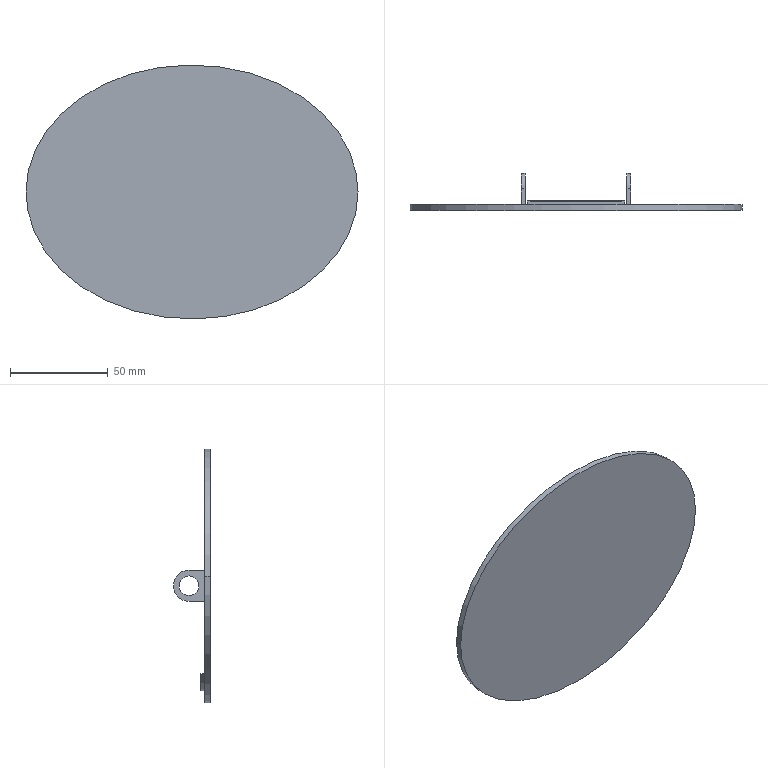Part | SolidWorks | features ICE 6, Extrusion 1, SweepCut 1 | 1 solid | 49 faces | box 170 x 19 x 130 mm | volume 53107 mm3 | plane 26 | cylinder 19 | spline 2 | torus 2 | commonest cylinder face diameters 1.5 x5 10 x4 16 x2 80 x2 74 x1 75 x1
STEP:
#1=CARTESIAN_POINT('',(0.,5.,-58.775));
#2=VERTEX_POINT('',#1);
#3=CARTESIAN_POINT('',(-25.,5.,-50.));
#4=VERTEX_POINT('',#3);
#5=CARTESIAN_POINT('',(0.,5.,-18.775));
#6=DIRECTION('',(0.,1.,0.));
#7=DIRECTION('',(0.,0.,-1.));
#8=AXIS2_PLACEMENT_3D('',#5,#6,#7);
#9=CIRCLE('',#8,40.);
#10=EDGE_CURVE('',#2,#4,#9,.T.);
#11=ORIENTED_EDGE('',*,*,#10,.F.);
#12=CARTESIAN_POINT('',(0.,3.,-58.775));
#13=VERTEX_POINT('',#12);
#14=CARTESIAN_POINT('',(0.,5.,-58.775));
#15=DIRECTION('',(0.,-1.,0.));
#16=VECTOR('',#15,1000.);
#17=LINE('',#14,#16);
#18=EDGE_CURVE('',#2,#13,#17,.T.);
#19=ORIENTED_EDGE('',*,*,#18,.T.);
#20=CARTESIAN_POINT('',(-25.,3.,-50.));
#21=VERTEX_POINT('',#20);
#22=CARTESIAN_POINT('',(0.,3.,-18.775));
#23=DIRECTION('',(0.,1.,0.));
#24=DIRECTION('',(0.,0.,-1.));
#25=AXIS2_PLACEMENT_3D('',#22,#23,#24);
#26=CIRCLE('',#25,40.);
#27=EDGE_CURVE('',#13,#21,#26,.T.);
#28=ORIENTED_EDGE('',*,*,#27,.T.);
#29=CARTESIAN_POINT('',(-25.,5.,-50.));
#30=DIRECTION('',(0.,-1.,0.));
#31=VECTOR('',#30,1000.);
#32=LINE('',#29,#31);
#33=EDGE_CURVE('',#4,#21,#32,.T.);
#34=ORIENTED_EDGE('',*,*,#33,.F.);
#35=EDGE_LOOP('',(#11,#19,#28,#34));
#36=FACE_OUTER_BOUND('',#35,.T.);
#37=CARTESIAN_POINT('',(0.,5.,-18.775));
#38=DIRECTION('',(0.,-1.,0.));
#39=DIRECTION('',(0.,0.,-1.));
#40=AXIS2_PLACEMENT_3D('',#37,#38,#39);
#41=CYLINDRICAL_SURFACE('',#40,40.);
#42=ADVANCED_FACE('',(#36),#41,.T.);
#43=CARTESIAN_POINT('',(-26.,11.,0.));
#44=VERTEX_POINT('',#43);
#45=CARTESIAN_POINT('',(-26.,11.,-10.));
#46=VERTEX_POINT('',#45);
#47=CARTESIAN_POINT('',(-26.,11.,-5.));
#48=DIRECTION('',(1.,0.,0.));
#49=DIRECTION('',(0.,0.,-1.));
#50=AXIS2_PLACEMENT_3D('',#47,#48,#49);
#51=CIRCLE('',#50,5.);
#52=EDGE_CURVE('',#44,#46,#51,.T.);
#53=ORIENTED_EDGE('',*,*,#52,.T.);
#54=CARTESIAN_POINT('',(-28.,11.,-10.));
#55=VERTEX_POINT('',#54);
#56=CARTESIAN_POINT('',(-26.,11.,-10.));
#57=DIRECTION('',(-1.,0.,0.));
#58=VECTOR('',#57,1000.);
#59=LINE('',#56,#58);
#60=EDGE_CURVE('',#46,#55,#59,.T.);
#61=ORIENTED_EDGE('',*,*,#60,.T.);
#62=CARTESIAN_POINT('',(-28.,11.,0.));
#63=VERTEX_POINT('',#62);
#64=CARTESIAN_POINT('',(-28.,11.,-5.));
#65=DIRECTION('',(1.,0.,0.));
#66=DIRECTION('',(0.,0.,-1.));
#67=AXIS2_PLACEMENT_3D('',#64,#65,#66);
#68=CIRCLE('',#67,5.);
#69=EDGE_CURVE('',#63,#55,#68,.T.);
#70=ORIENTED_EDGE('',*,*,#69,.F.);
#71=CARTESIAN_POINT('',(-26.,11.,0.));
#72=DIRECTION('',(-1.,0.,0.));
#73=VECTOR('',#72,1000.);
#74=LINE('',#71,#73);
#75=EDGE_CURVE('',#44,#63,#74,.T.);
#76=ORIENTED_EDGE('',*,*,#75,.F.);
#77=EDGE_LOOP('',(#53,#61,#70,#76));
#78=FACE_OUTER_BOUND('',#77,.T.);
#79=CARTESIAN_POINT('',(-26.,11.,-5.));
#80=DIRECTION('',(-1.,0.,0.));
#81=DIRECTION('',(0.,0.,1.));
#82=AXIS2_PLACEMENT_3D('',#79,#80,#81);
#83=CYLINDRICAL_SURFACE('',#82,5.);
#84=ADVANCED_FACE('',(#78),#83,.F.);
#85=CARTESIAN_POINT('',(26.,11.,0.));
#86=VERTEX_POINT('',#85);
#87=CARTESIAN_POINT('',(26.,11.,-10.));
#88=VERTEX_POINT('',#87);
#89=CARTESIAN_POINT('',(26.,11.,-5.));
#90=DIRECTION('',(1.,0.,0.));
#91=DIRECTION('',(0.,0.,-1.));
#92=AXIS2_PLACEMENT_3D('',#89,#90,#91);
#93=CIRCLE('',#92,5.);
#94=EDGE_CURVE('',#86,#88,#93,.T.);
#95=ORIENTED_EDGE('',*,*,#94,.F.);
#96=CARTESIAN_POINT('',(28.,11.,0.));
#97=VERTEX_POINT('',#96);
#98=CARTESIAN_POINT('',(26.,11.,0.));
#99=DIRECTION('',(1.,0.,0.));
#100=VECTOR('',#99,1000.);
#101=LINE('',#98,#100);
#102=EDGE_CURVE('',#86,#97,#101,.T.);
#103=ORIENTED_EDGE('',*,*,#102,.T.);
#104=CARTESIAN_POINT('',(28.,11.,-10.));
#105=VERTEX_POINT('',#104);
#106=CARTESIAN_POINT('',(28.,11.,-5.));
#107=DIRECTION('',(1.,0.,0.));
#108=DIRECTION('',(0.,0.,-1.));
#109=AXIS2_PLACEMENT_3D('',#106,#107,#108);
#110=CIRCLE('',#109,5.);
#111=EDGE_CURVE('',#97,#105,#110,.T.);
#112=ORIENTED_EDGE('',*,*,#111,.T.);
#113=CARTESIAN_POINT('',(26.,11.,-10.));
#114=DIRECTION('',(1.,0.,0.));
#115=VECTOR('',#114,1000.);
#116=LINE('',#113,#115);
#117=EDGE_CURVE('',#88,#105,#116,.T.);
#118=ORIENTED_EDGE('',*,*,#117,.F.);
#119=EDGE_LOOP('',(#95,#103,#112,#118));
#120=FACE_OUTER_BOUND('',#119,.T.);
#121=CARTESIAN_POINT('',(26.,11.,-5.));
#122=DIRECTION('',(1.,0.,0.));
#123=DIRECTION('',(0.,0.,-1.));
#124=AXIS2_PLACEMENT_3D('',#121,#122,#123);
#125=CYLINDRICAL_SURFACE('',#124,5.);
#126=ADVANCED_FACE('',(#120),#125,.F.);
#127=CARTESIAN_POINT('',(85.,3.,0.));
#128=VERTEX_POINT('',#127);
#129=CARTESIAN_POINT('',(-85.,3.,0.));
#130=VERTEX_POINT('',#129);
#131=CARTESIAN_POINT('',(85.,3.,0.));
#132=CARTESIAN_POINT('',(85.,3.,-130.));
#133=CARTESIAN_POINT('',(-85.,3.,-130.));
#134=CARTESIAN_POINT('',(-85.,3.,0.));
#135=(BOUNDED_CURVE()B_SPLINE_CURVE(3,(#131,#132,#133,#134),.UNSPECIFIED.,.F.,.T.)B_SPLINE_CURVE_WITH_KNOTS((4,4),(3.142,6.283),.UNSPECIFIED.)CURVE()GEOMETRIC_REPRESENTATION_ITEM()RATIONAL_B_SPLINE_CURVE((1.,0.3333,0.3333,1.))REPRESENTATION_ITEM(''));
#136=EDGE_CURVE('',#128,#130,#135,.T.);
#137=ORIENTED_EDGE('',*,*,#136,.F.);
#138=CARTESIAN_POINT('',(85.,0.,0.));
#139=VERTEX_POINT('',#138);
#140=CARTESIAN_POINT('',(85.,3.,0.));
#141=DIRECTION('',(0.,-1.,0.));
#142=VECTOR('',#141,1000.);
#143=LINE('',#140,#142);
#144=EDGE_CURVE('',#128,#139,#143,.T.);
#145=ORIENTED_EDGE('',*,*,#144,.T.);
#146=CARTESIAN_POINT('',(-85.,0.,0.));
#147=VERTEX_POINT('',#146);
#148=CARTESIAN_POINT('',(85.,0.,0.));
#149=CARTESIAN_POINT('',(85.,0.,-130.));
#150=CARTESIAN_POINT('',(-85.,0.,-130.));
#151=CARTESIAN_POINT('',(-85.,0.,0.));
#152=(BOUNDED_CURVE()B_SPLINE_CURVE(3,(#148,#149,#150,#151),.UNSPECIFIED.,.F.,.T.)B_SPLINE_CURVE_WITH_KNOTS((4,4),(3.142,6.283),.UNSPECIFIED.)CURVE()GEOMETRIC_REPRESENTATION_ITEM()RATIONAL_B_SPLINE_CURVE((1.,0.3333,0.3333,1.))REPRESENTATION_ITEM(''));
#153=EDGE_CURVE('',#139,#147,#152,.T.);
#154=ORIENTED_EDGE('',*,*,#153,.T.);
#155=CARTESIAN_POINT('',(-85.,3.,0.));
#156=DIRECTION('',(0.,-1.,0.));
#157=VECTOR('',#156,1000.);
#158=LINE('',#155,#157);
#159=EDGE_CURVE('',#130,#147,#158,.T.);
#160=ORIENTED_EDGE('',*,*,#159,.F.);
#161=EDGE_LOOP('',(#137,#145,#154,#160));
#162=FACE_OUTER_BOUND('',#161,.T.);
#163=CARTESIAN_POINT('',(85.,3.,0.));
#164=CARTESIAN_POINT('',(85.,0.,0.));
#165=CARTESIAN_POINT('',(85.,3.,-130.));
#166=CARTESIAN_POINT('',(85.,0.,-130.));
#167=CARTESIAN_POINT('',(-85.,3.,-130.));
#168=CARTESIAN_POINT('',(-85.,0.,-130.));
#169=CARTESIAN_POINT('',(-85.,3.,0.));
#170=CARTESIAN_POINT('',(-85.,0.,0.));
#171=(BOUNDED_SURFACE()B_SPLINE_SURFACE(3,1,((#163,#164),(#165,#166),(#167,#168),(#169,#170)),.UNSPECIFIED.,.F.,.F.,.T.)B_SPLINE_SURFACE_WITH_KNOTS((4,4),(2,2),(0.,1.),(0.,1.),.UNSPECIFIED.)GEOMETRIC_REPRESENTATION_ITEM()RATIONAL_B_SPLINE_SURFACE(((1.,1.),(0.3333,0.3333),(0.3333,0.3333),(1.,1.)))REPRESENTATION_ITEM('')SURFACE());
#172=ADVANCED_FACE('',(#162),#171,.F.);
#173=CARTESIAN_POINT('',(26.,3.,3.));
#174=VERTEX_POINT('',#173);
#175=CARTESIAN_POINT('',(26.,3.,-13.));
#176=VERTEX_POINT('',#175);
#177=CARTESIAN_POINT('',(26.,3.,-13.));
#178=DIRECTION('',(0.,0.,-1.));
#179=VECTOR('',#178,1000.);
#180=LINE('',#177,#179);
#181=EDGE_CURVE('',#174,#176,#180,.T.);
#182=ORIENTED_EDGE('',*,*,#181,.T.);
#183=CARTESIAN_POINT('',(28.,3.,-13.));
#184=VERTEX_POINT('',#183);
#185=CARTESIAN_POINT('',(26.,3.,-13.));
#186=DIRECTION('',(1.,0.,0.));
#187=VECTOR('',#186,1000.);
#188=LINE('',#185,#187);
#189=EDGE_CURVE('',#176,#184,#188,.T.);
#190=ORIENTED_EDGE('',*,*,#189,.T.);
#191=CARTESIAN_POINT('',(28.,3.,3.));
#192=VERTEX_POINT('',#191);
#193=CARTESIAN_POINT('',(28.,3.,-13.));
#194=DIRECTION('',(0.,0.,-1.));
#195=VECTOR('',#194,1000.);
#196=LINE('',#193,#195);
#197=EDGE_CURVE('',#192,#184,#196,.T.);
#198=ORIENTED_EDGE('',*,*,#197,.F.);
#199=CARTESIAN_POINT('',(26.,3.,3.));
#200=DIRECTION('',(1.,0.,0.));
#201=VECTOR('',#200,1000.);
#202=LINE('',#199,#201);
#203=EDGE_CURVE('',#174,#192,#202,.T.);
#204=ORIENTED_EDGE('',*,*,#203,.F.);
#205=EDGE_LOOP('',(#182,#190,#198,#204));
#206=FACE_BOUND('',#205,.T.);
#207=CARTESIAN_POINT('',(-85.,3.,0.));
#208=CARTESIAN_POINT('',(-85.,3.,130.));
#209=CARTESIAN_POINT('',(85.,3.,130.));
#210=CARTESIAN_POINT('',(85.,3.,0.));
#211=(BOUNDED_CURVE()B_SPLINE_CURVE(3,(#207,#208,#209,#210),.UNSPECIFIED.,.F.,.T.)B_SPLINE_CURVE_WITH_KNOTS((4,4),(0.,3.142),.UNSPECIFIED.)CURVE()GEOMETRIC_REPRESENTATION_ITEM()RATIONAL_B_SPLINE_CURVE((1.,0.3333,0.3333,1.))REPRESENTATION_ITEM(''));
#212=EDGE_CURVE('',#130,#128,#211,.T.);
#213=ORIENTED_EDGE('',*,*,#212,.T.);
#214=ORIENTED_EDGE('',*,*,#136,.T.);
#215=EDGE_LOOP('',(#213,#214));
#216=FACE_OUTER_BOUND('',#215,.T.);
#217=CARTESIAN_POINT('',(-28.,3.,3.));
#218=VERTEX_POINT('',#217);
#219=CARTESIAN_POINT('',(-28.,3.,-13.));
#220=VERTEX_POINT('',#219);
#221=CARTESIAN_POINT('',(-28.,3.,-13.));
#222=DIRECTION('',(0.,0.,-1.));
#223=VECTOR('',#222,1000.);
#224=LINE('',#221,#223);
#225=EDGE_CURVE('',#218,#220,#224,.T.);
#226=ORIENTED_EDGE('',*,*,#225,.T.);
#227=CARTESIAN_POINT('',(-26.,3.,-13.));
#228=VERTEX_POINT('',#227);
#229=CARTESIAN_POINT('',(-26.,3.,-13.));
#230=DIRECTION('',(-1.,0.,0.));
#231=VECTOR('',#230,1000.);
#232=LINE('',#229,#231);
#233=EDGE_CURVE('',#228,#220,#232,.T.);
#234=ORIENTED_EDGE('',*,*,#233,.F.);
#235=CARTESIAN_POINT('',(-26.,3.,3.));
#236=VERTEX_POINT('',#235);
#237=CARTESIAN_POINT('',(-26.,3.,-13.));
#238=DIRECTION('',(0.,0.,-1.));
#239=VECTOR('',#238,1000.);
#240=LINE('',#237,#239);
#241=EDGE_CURVE('',#236,#228,#240,.T.);
#242=ORIENTED_EDGE('',*,*,#241,.F.);
#243=CARTESIAN_POINT('',(-26.,3.,3.));
#244=DIRECTION('',(-1.,0.,0.));
#245=VECTOR('',#244,1000.);
#246=LINE('',#243,#245);
#247=EDGE_CURVE('',#236,#218,#246,.T.);
#248=ORIENTED_EDGE('',*,*,#247,.T.);
#249=EDGE_LOOP('',(#226,#234,#242,#248));
#250=FACE_BOUND('',#249,.T.);
#251=CARTESIAN_POINT('',(-15.75,3.,30.));
#252=VERTEX_POINT('',#251);
#253=CARTESIAN_POINT('',(-15.75,3.,-5.));
#254=VERTEX_POINT('',#253);
#255=CARTESIAN_POINT('',(-15.75,3.,-5.));
#256=DIRECTION('',(0.,0.,-1.));
#257=VECTOR('',#256,1000.);
#258=LINE('',#255,#257);
#259=EDGE_CURVE('',#252,#254,#258,.T.);
#260=ORIENTED_EDGE('',*,*,#259,.T.);
#261=CARTESIAN_POINT('',(-15.75,3.,-10.));
#262=VERTEX_POINT('',#261);
#263=CARTESIAN_POINT('',(-15.75,3.,-10.));
#264=DIRECTION('',(0.,0.,-1.));
#265=VECTOR('',#264,1000.);
#266=LINE('',#263,#265);
#267=EDGE_CURVE('',#254,#262,#266,.T.);
#268=ORIENTED_EDGE('',*,*,#267,.T.);
#269=CARTESIAN_POINT('',(-14.25,3.,-10.));
#270=VERTEX_POINT('',#269);
#271=CARTESIAN_POINT('',(0.,3.,-10.));
#272=DIRECTION('',(-1.,0.,0.));
#273=VECTOR('',#272,1000.);
#274=LINE('',#271,#273);
#275=EDGE_CURVE('',#270,#262,#274,.T.);
#276=ORIENTED_EDGE('',*,*,#275,.F.);
#277=CARTESIAN_POINT('',(-14.25,3.,-5.));
#278=VERTEX_POINT('',#277);
#279=CARTESIAN_POINT('',(-14.25,3.,-10.));
#280=DIRECTION('',(0.,0.,1.));
#281=VECTOR('',#280,1000.);
#282=LINE('',#279,#281);
#283=EDGE_CURVE('',#270,#278,#282,.T.);
#284=ORIENTED_EDGE('',*,*,#283,.T.);
#285=CARTESIAN_POINT('',(-14.25,3.,30.));
#286=VERTEX_POINT('',#285);
#287=CARTESIAN_POINT('',(-14.25,3.,-5.));
#288=DIRECTION('',(0.,0.,1.));
#289=VECTOR('',#288,1000.);
#290=LINE('',#287,#289);
#291=EDGE_CURVE('',#278,#286,#290,.T.);
#292=ORIENTED_EDGE('',*,*,#291,.T.);
#293=CARTESIAN_POINT('',(-10.,3.,34.25));
#294=VERTEX_POINT('',#293);
#295=CARTESIAN_POINT('',(-10.,3.,30.));
#296=DIRECTION('',(0.,1.,0.));
#297=DIRECTION('',(0.,0.,-1.));
#298=AXIS2_PLACEMENT_3D('',#295,#296,#297);
#299=CIRCLE('',#298,4.25);
#300=EDGE_CURVE('',#286,#294,#299,.T.);
#301=ORIENTED_EDGE('',*,*,#300,.T.);
#302=CARTESIAN_POINT('',(10.,3.,34.25));
#303=VERTEX_POINT('',#302);
#304=CARTESIAN_POINT('',(-10.,3.,34.25));
#305=DIRECTION('',(1.,0.,0.));
#306=VECTOR('',#305,1000.);
#307=LINE('',#304,#306);
#308=EDGE_CURVE('',#294,#303,#307,.T.);
#309=ORIENTED_EDGE('',*,*,#308,.T.);
#310=CARTESIAN_POINT('',(14.25,3.,30.));
#311=VERTEX_POINT('',#310);
#312=CARTESIAN_POINT('',(10.,3.,30.));
#313=DIRECTION('',(0.,1.,0.));
#314=DIRECTION('',(0.,0.,-1.));
#315=AXIS2_PLACEMENT_3D('',#312,#313,#314);
#316=CIRCLE('',#315,4.25);
#317=EDGE_CURVE('',#303,#311,#316,.T.);
#318=ORIENTED_EDGE('',*,*,#317,.T.);
#319=CARTESIAN_POINT('',(14.25,3.,-5.));
#320=VERTEX_POINT('',#319);
#321=CARTESIAN_POINT('',(14.25,3.,30.));
#322=DIRECTION('',(0.,0.,-1.));
#323=VECTOR('',#322,1000.);
#324=LINE('',#321,#323);
#325=EDGE_CURVE('',#311,#320,#324,.T.);
#326=ORIENTED_EDGE('',*,*,#325,.T.);
#327=CARTESIAN_POINT('',(14.25,3.,-10.));
#328=VERTEX_POINT('',#327);
#329=CARTESIAN_POINT('',(14.25,3.,-5.));
#330=DIRECTION('',(0.,0.,-1.));
#331=VECTOR('',#330,1000.);
#332=LINE('',#329,#331);
#333=EDGE_CURVE('',#320,#328,#332,.T.);
#334=ORIENTED_EDGE('',*,*,#333,.T.);
#335=CARTESIAN_POINT('',(15.75,3.,-10.));
#336=VERTEX_POINT('',#335);
#337=CARTESIAN_POINT('',(0.,3.,-10.));
#338=DIRECTION('',(1.,0.,0.));
#339=VECTOR('',#338,1000.);
#340=LINE('',#337,#339);
#341=EDGE_CURVE('',#328,#336,#340,.T.);
#342=ORIENTED_EDGE('',*,*,#341,.T.);
#343=CARTESIAN_POINT('',(15.75,3.,-5.));
#344=VERTEX_POINT('',#343);
#345=CARTESIAN_POINT('',(15.75,3.,-5.));
#346=DIRECTION('',(0.,0.,1.));
#347=VECTOR('',#346,1000.);
#348=LINE('',#345,#347);
#349=EDGE_CURVE('',#336,#344,#348,.T.);
#350=ORIENTED_EDGE('',*,*,#349,.T.);
#351=CARTESIAN_POINT('',(15.75,3.,30.));
#352=VERTEX_POINT('',#351);
#353=CARTESIAN_POINT('',(15.75,3.,30.));
#354=DIRECTION('',(0.,0.,1.));
#355=VECTOR('',#354,1000.);
#356=LINE('',#353,#355);
#357=EDGE_CURVE('',#344,#352,#356,.T.);
#358=ORIENTED_EDGE('',*,*,#357,.T.);
#359=CARTESIAN_POINT('',(10.,3.,35.75));
#360=VERTEX_POINT('',#359);
#361=CARTESIAN_POINT('',(10.,3.,30.));
#362=DIRECTION('',(0.,-1.,0.));
#363=DIRECTION('',(0.,0.,1.));
#364=AXIS2_PLACEMENT_3D('',#361,#362,#363);
#365=CIRCLE('',#364,5.75);
#366=EDGE_CURVE('',#352,#360,#365,.T.);
#367=ORIENTED_EDGE('',*,*,#366,.T.);
#368=CARTESIAN_POINT('',(-10.,3.,35.75));
#369=VERTEX_POINT('',#368);
#370=CARTESIAN_POINT('',(-10.,3.,35.75));
#371=DIRECTION('',(-1.,0.,0.));
#372=VECTOR('',#371,1000.);
#373=LINE('',#370,#372);
#374=EDGE_CURVE('',#360,#369,#373,.T.);
#375=ORIENTED_EDGE('',*,*,#374,.T.);
#376=CARTESIAN_POINT('',(-10.,3.,30.));
#377=DIRECTION('',(0.,-1.,0.));
#378=DIRECTION('',(0.,0.,1.));
#379=AXIS2_PLACEMENT_3D('',#376,#377,#378);
#380=CIRCLE('',#379,5.75);
#381=EDGE_CURVE('',#369,#252,#380,.T.);
#382=ORIENTED_EDGE('',*,*,#381,.T.);
#383=EDGE_LOOP('',(#260,#268,#276,#284,#292,#301,#309,#318,#326,#334,#342,#350,#358,#367,#375,#382));
#384=FACE_BOUND('',#383,.T.);
#385=CARTESIAN_POINT('',(25.,3.,-50.));
#386=VERTEX_POINT('',#385);
#387=CARTESIAN_POINT('',(-25.,3.,-50.));
#388=DIRECTION('',(1.,0.,0.));
#389=VECTOR('',#388,1000.);
#390=LINE('',#387,#389);
#391=EDGE_CURVE('',#21,#386,#390,.T.);
#392=ORIENTED_EDGE('',*,*,#391,.F.);
#393=ORIENTED_EDGE('',*,*,#27,.F.);
#394=CARTESIAN_POINT('',(0.,3.,-18.775));
#395=DIRECTION('',(0.,1.,0.));
#396=DIRECTION('',(0.,0.,-1.));
#397=AXIS2_PLACEMENT_3D('',#394,#395,#396);
#398=CIRCLE('',#397,40.);
#399=EDGE_CURVE('',#386,#13,#398,.T.);
#400=ORIENTED_EDGE('',*,*,#399,.F.);
#401=EDGE_LOOP('',(#392,#393,#400));
#402=FACE_BOUND('',#401,.T.);
#403=CARTESIAN_POINT('',(0.,3.,0.));
#404=DIRECTION('',(0.,1.,0.));
#405=DIRECTION('',(0.,0.,1.));
#406=AXIS2_PLACEMENT_3D('',#403,#404,#405);
#407=PLANE('',#406);
#408=ADVANCED_FACE('',(#206,#216,#250,#384,#402),#407,.T.);
#409=ORIENTED_EDGE('',*,*,#144,.F.);
#410=ORIENTED_EDGE('',*,*,#212,.F.);
#411=ORIENTED_EDGE('',*,*,#159,.T.);
#412=CARTESIAN_POINT('',(-85.,0.,0.));
#413=CARTESIAN_POINT('',(-85.,0.,130.));
#414=CARTESIAN_POINT('',(85.,0.,130.));
#415=CARTESIAN_POINT('',(85.,0.,0.));
#416=(BOUNDED_CURVE()B_SPLINE_CURVE(3,(#412,#413,#414,#415),.UNSPECIFIED.,.F.,.F.)B_SPLINE_CURVE_WITH_KNOTS((4,4),(0.,3.142),.UNSPECIFIED.)CURVE()GEOMETRIC_REPRESENTATION_ITEM()RATIONAL_B_SPLINE_CURVE((1.,0.3333,0.3333,1.))REPRESENTATION_ITEM(''));
#417=EDGE_CURVE('',#147,#139,#416,.T.);
#418=ORIENTED_EDGE('',*,*,#417,.T.);
#419=EDGE_LOOP('',(#409,#410,#411,#418));
#420=FACE_OUTER_BOUND('',#419,.T.);
#421=CARTESIAN_POINT('',(-85.,3.,0.));
#422=CARTESIAN_POINT('',(-85.,0.,0.));
#423=CARTESIAN_POINT('',(-85.,3.,130.));
#424=CARTESIAN_POINT('',(-85.,0.,130.));
#425=CARTESIAN_POINT('',(85.,3.,130.));
#426=CARTESIAN_POINT('',(85.,0.,130.));
#427=CARTESIAN_POINT('',(85.,3.,0.));
#428=CARTESIAN_POINT('',(85.,0.,0.));
#429=(BOUNDED_SURFACE()B_SPLINE_SURFACE(3,1,((#421,#422),(#423,#424),(#425,#426),(#427,#428)),.UNSPECIFIED.,.F.,.F.,.T.)B_SPLINE_SURFACE_WITH_KNOTS((4,4),(2,2),(0.,1.),(0.,1.),.UNSPECIFIED.)GEOMETRIC_REPRESENTATION_ITEM()RATIONAL_B_SPLINE_SURFACE(((1.,1.),(0.3333,0.3333),(0.3333,0.3333),(1.,1.)))REPRESENTATION_ITEM('')SURFACE());
#430=ADVANCED_FACE('',(#420),#429,.F.);
#431=ORIENTED_EDGE('',*,*,#417,.F.);
#432=ORIENTED_EDGE('',*,*,#153,.F.);
#433=EDGE_LOOP('',(#431,#432));
#434=FACE_OUTER_BOUND('',#433,.T.);
#435=CARTESIAN_POINT('',(0.,0.,0.));
#436=DIRECTION('',(0.,1.,0.));
#437=DIRECTION('',(0.,0.,1.));
#438=AXIS2_PLACEMENT_3D('',#435,#436,#437);
#439=PLANE('',#438);
#440=ADVANCED_FACE('',(#434),#439,.F.);
#441=CARTESIAN_POINT('',(28.,11.,3.));
#442=VERTEX_POINT('',#441);
#443=CARTESIAN_POINT('',(28.,3.,3.));
#444=DIRECTION('',(0.,-1.,0.));
#445=VECTOR('',#444,1000.);
#446=LINE('',#443,#445);
#447=EDGE_CURVE('',#442,#192,#446,.T.);
#448=ORIENTED_EDGE('',*,*,#447,.F.);
#449=CARTESIAN_POINT('',(26.,11.,3.));
#450=VERTEX_POINT('',#449);
#451=CARTESIAN_POINT('',(26.,11.,3.));
#452=DIRECTION('',(1.,0.,0.));
#453=VECTOR('',#452,1000.);
#454=LINE('',#451,#453);
#455=EDGE_CURVE('',#450,#442,#454,.T.);
#456=ORIENTED_EDGE('',*,*,#455,.F.);
#457=CARTESIAN_POINT('',(26.,3.,3.));
#458=DIRECTION('',(0.,-1.,0.));
#459=VECTOR('',#458,1000.);
#460=LINE('',#457,#459);
#461=EDGE_CURVE('',#450,#174,#460,.T.);
#462=ORIENTED_EDGE('',*,*,#461,.T.);
#463=ORIENTED_EDGE('',*,*,#203,.T.);
#464=EDGE_LOOP('',(#448,#456,#462,#463));
#465=FACE_OUTER_BOUND('',#464,.T.);
#466=CARTESIAN_POINT('',(26.,3.,3.));
#467=DIRECTION('',(0.,0.,1.));
#468=DIRECTION('',(1.,0.,0.));
#469=AXIS2_PLACEMENT_3D('',#466,#467,#468);
#470=PLANE('',#469);
#471=ADVANCED_FACE('',(#465),#470,.T.);
#472=CARTESIAN_POINT('',(28.,11.,-13.));
#473=VERTEX_POINT('',#472);
#474=CARTESIAN_POINT('',(28.,11.,-5.));
#475=DIRECTION('',(1.,0.,0.));
#476=DIRECTION('',(0.,0.,1.));
#477=AXIS2_PLACEMENT_3D('',#474,#475,#476);
#478=CIRCLE('',#477,8.);
#479=EDGE_CURVE('',#473,#442,#478,.T.);
#480=ORIENTED_EDGE('',*,*,#479,.F.);
#481=CARTESIAN_POINT('',(26.,11.,-13.));
#482=VERTEX_POINT('',#481);
#483=CARTESIAN_POINT('',(26.,11.,-13.));
#484=DIRECTION('',(1.,0.,0.));
#485=VECTOR('',#484,1000.);
#486=LINE('',#483,#485);
#487=EDGE_CURVE('',#482,#473,#486,.T.);
#488=ORIENTED_EDGE('',*,*,#487,.F.);
#489=CARTESIAN_POINT('',(26.,11.,-5.));
#490=DIRECTION('',(1.,0.,0.));
#491=DIRECTION('',(0.,0.,1.));
#492=AXIS2_PLACEMENT_3D('',#489,#490,#491);
#493=CIRCLE('',#492,8.);
#494=EDGE_CURVE('',#482,#450,#493,.T.);
#495=ORIENTED_EDGE('',*,*,#494,.T.);
#496=ORIENTED_EDGE('',*,*,#455,.T.);
#497=EDGE_LOOP('',(#480,#488,#495,#496));
#498=FACE_OUTER_BOUND('',#497,.T.);
#499=CARTESIAN_POINT('',(26.,11.,-5.));
#500=DIRECTION('',(1.,0.,0.));
#501=DIRECTION('',(0.,0.,-1.));
#502=AXIS2_PLACEMENT_3D('',#499,#500,#501);
#503=CYLINDRICAL_SURFACE('',#502,8.);
#504=ADVANCED_FACE('',(#498),#503,.T.);
#505=CARTESIAN_POINT('',(28.,11.,-13.));
#506=DIRECTION('',(0.,1.,0.));
#507=VECTOR('',#506,1000.);
#508=LINE('',#505,#507);
#509=EDGE_CURVE('',#184,#473,#508,.T.);
#510=ORIENTED_EDGE('',*,*,#509,.F.);
#511=ORIENTED_EDGE('',*,*,#189,.F.);
#512=CARTESIAN_POINT('',(26.,11.,-13.));
#513=DIRECTION('',(0.,1.,0.));
#514=VECTOR('',#513,1000.);
#515=LINE('',#512,#514);
#516=EDGE_CURVE('',#176,#482,#515,.T.);
#517=ORIENTED_EDGE('',*,*,#516,.T.);
#518=ORIENTED_EDGE('',*,*,#487,.T.);
#519=EDGE_LOOP('',(#510,#511,#517,#518));
#520=FACE_OUTER_BOUND('',#519,.T.);
#521=CARTESIAN_POINT('',(26.,11.,-13.));
#522=DIRECTION('',(0.,0.,-1.));
#523=DIRECTION('',(-1.,0.,0.));
#524=AXIS2_PLACEMENT_3D('',#521,#522,#523);
#525=PLANE('',#524);
#526=ADVANCED_FACE('',(#520),#525,.T.);
#527=CARTESIAN_POINT('',(26.,11.,-5.));
#528=DIRECTION('',(1.,0.,0.));
#529=DIRECTION('',(0.,0.,-1.));
#530=AXIS2_PLACEMENT_3D('',#527,#528,#529);
#531=CIRCLE('',#530,5.);
#532=EDGE_CURVE('',#88,#86,#531,.T.);
#533=ORIENTED_EDGE('',*,*,#532,.T.);
#534=ORIENTED_EDGE('',*,*,#94,.T.);
#535=EDGE_LOOP('',(#533,#534));
#536=FACE_BOUND('',#535,.T.);
#537=ORIENTED_EDGE('',*,*,#181,.F.);
#538=ORIENTED_EDGE('',*,*,#461,.F.);
#539=ORIENTED_EDGE('',*,*,#494,.F.);
#540=ORIENTED_EDGE('',*,*,#516,.F.);
#541=EDGE_LOOP('',(#537,#538,#539,#540));
#542=FACE_OUTER_BOUND('',#541,.T.);
#543=CARTESIAN_POINT('',(26.,11.,-5.));
#544=DIRECTION('',(-1.,0.,0.));
#545=DIRECTION('',(0.,0.,1.));
#546=AXIS2_PLACEMENT_3D('',#543,#544,#545);
#547=PLANE('',#546);
#548=ADVANCED_FACE('',(#536,#542),#547,.T.);
#549=CARTESIAN_POINT('',(28.,11.,-5.));
#550=DIRECTION('',(1.,0.,0.));
#551=DIRECTION('',(0.,0.,-1.));
#552=AXIS2_PLACEMENT_3D('',#549,#550,#551);
#553=CIRCLE('',#552,5.);
#554=EDGE_CURVE('',#105,#97,#553,.T.);
#555=ORIENTED_EDGE('',*,*,#554,.F.);
#556=ORIENTED_EDGE('',*,*,#111,.F.);
#557=EDGE_LOOP('',(#555,#556));
#558=FACE_BOUND('',#557,.T.);
#559=ORIENTED_EDGE('',*,*,#197,.T.);
#560=ORIENTED_EDGE('',*,*,#509,.T.);
#561=ORIENTED_EDGE('',*,*,#479,.T.);
#562=ORIENTED_EDGE('',*,*,#447,.T.);
#563=EDGE_LOOP('',(#559,#560,#561,#562));
#564=FACE_OUTER_BOUND('',#563,.T.);
#565=CARTESIAN_POINT('',(28.,11.,-5.));
#566=DIRECTION('',(-1.,0.,0.));
#567=DIRECTION('',(0.,0.,1.));
#568=AXIS2_PLACEMENT_3D('',#565,#566,#567);
#569=PLANE('',#568);
#570=ADVANCED_FACE('',(#558,#564),#569,.F.);
#571=ORIENTED_EDGE('',*,*,#102,.F.);
#572=ORIENTED_EDGE('',*,*,#532,.F.);
#573=ORIENTED_EDGE('',*,*,#117,.T.);
#574=ORIENTED_EDGE('',*,*,#554,.T.);
#575=EDGE_LOOP('',(#571,#572,#573,#574));
#576=FACE_OUTER_BOUND('',#575,.T.);
#577=CARTESIAN_POINT('',(26.,11.,-5.));
#578=DIRECTION('',(1.,0.,0.));
#579=DIRECTION('',(0.,0.,-1.));
#580=AXIS2_PLACEMENT_3D('',#577,#578,#579);
#581=CYLINDRICAL_SURFACE('',#580,5.);
#582=ADVANCED_FACE('',(#576),#581,.F.);
#583=ORIENTED_EDGE('',*,*,#241,.T.);
#584=CARTESIAN_POINT('',(-26.,11.,-13.));
#585=VERTEX_POINT('',#584);
#586=CARTESIAN_POINT('',(-26.,11.,-13.));
#587=DIRECTION('',(0.,1.,0.));
#588=VECTOR('',#587,1000.);
#589=LINE('',#586,#588);
#590=EDGE_CURVE('',#228,#585,#589,.T.);
#591=ORIENTED_EDGE('',*,*,#590,.T.);
#592=CARTESIAN_POINT('',(-26.,11.,3.));
#593=VERTEX_POINT('',#592);
#594=CARTESIAN_POINT('',(-26.,11.,-5.));
#595=DIRECTION('',(1.,0.,0.));
#596=DIRECTION('',(0.,0.,1.));
#597=AXIS2_PLACEMENT_3D('',#594,#595,#596);
#598=CIRCLE('',#597,8.);
#599=EDGE_CURVE('',#585,#593,#598,.T.);
#600=ORIENTED_EDGE('',*,*,#599,.T.);
#601=CARTESIAN_POINT('',(-26.,3.,3.));
#602=DIRECTION('',(0.,-1.,0.));
#603=VECTOR('',#602,1000.);
#604=LINE('',#601,#603);
#605=EDGE_CURVE('',#593,#236,#604,.T.);
#606=ORIENTED_EDGE('',*,*,#605,.T.);
#607=EDGE_LOOP('',(#583,#591,#600,#606));
#608=FACE_OUTER_BOUND('',#607,.T.);
#609=ORIENTED_EDGE('',*,*,#52,.F.);
#610=CARTESIAN_POINT('',(-26.,11.,-5.));
#611=DIRECTION('',(1.,0.,0.));
#612=DIRECTION('',(0.,0.,-1.));
#613=AXIS2_PLACEMENT_3D('',#610,#611,#612);
#614=CIRCLE('',#613,5.);
#615=EDGE_CURVE('',#46,#44,#614,.T.);
#616=ORIENTED_EDGE('',*,*,#615,.F.);
#617=EDGE_LOOP('',(#609,#616));
#618=FACE_BOUND('',#617,.T.);
#619=CARTESIAN_POINT('',(-26.,11.,-5.));
#620=DIRECTION('',(-1.,0.,0.));
#621=DIRECTION('',(0.,0.,1.));
#622=AXIS2_PLACEMENT_3D('',#619,#620,#621);
#623=PLANE('',#622);
#624=ADVANCED_FACE('',(#608,#618),#623,.F.);
#625=ORIENTED_EDGE('',*,*,#225,.F.);
#626=CARTESIAN_POINT('',(-28.,11.,3.));
#627=VERTEX_POINT('',#626);
#628=CARTESIAN_POINT('',(-28.,3.,3.));
#629=DIRECTION('',(0.,-1.,0.));
#630=VECTOR('',#629,1000.);
#631=LINE('',#628,#630);
#632=EDGE_CURVE('',#627,#218,#631,.T.);
#633=ORIENTED_EDGE('',*,*,#632,.F.);
#634=CARTESIAN_POINT('',(-28.,11.,-13.));
#635=VERTEX_POINT('',#634);
#636=CARTESIAN_POINT('',(-28.,11.,-5.));
#637=DIRECTION('',(1.,0.,0.));
#638=DIRECTION('',(0.,0.,1.));
#639=AXIS2_PLACEMENT_3D('',#636,#637,#638);
#640=CIRCLE('',#639,8.);
#641=EDGE_CURVE('',#635,#627,#640,.T.);
#642=ORIENTED_EDGE('',*,*,#641,.F.);
#643=CARTESIAN_POINT('',(-28.,11.,-13.));
#644=DIRECTION('',(0.,1.,0.));
#645=VECTOR('',#644,1000.);
#646=LINE('',#643,#645);
#647=EDGE_CURVE('',#220,#635,#646,.T.);
#648=ORIENTED_EDGE('',*,*,#647,.F.);
#649=EDGE_LOOP('',(#625,#633,#642,#648));
#650=FACE_OUTER_BOUND('',#649,.T.);
#651=ORIENTED_EDGE('',*,*,#69,.T.);
#652=CARTESIAN_POINT('',(-28.,11.,-5.));
#653=DIRECTION('',(1.,0.,0.));
#654=DIRECTION('',(0.,0.,-1.));
#655=AXIS2_PLACEMENT_3D('',#652,#653,#654);
#656=CIRCLE('',#655,5.);
#657=EDGE_CURVE('',#55,#63,#656,.T.);
#658=ORIENTED_EDGE('',*,*,#657,.T.);
#659=EDGE_LOOP('',(#651,#658));
#660=FACE_BOUND('',#659,.T.);
#661=CARTESIAN_POINT('',(-28.,11.,-5.));
#662=DIRECTION('',(-1.,0.,0.));
#663=DIRECTION('',(0.,0.,1.));
#664=AXIS2_PLACEMENT_3D('',#661,#662,#663);
#665=PLANE('',#664);
#666=ADVANCED_FACE('',(#650,#660),#665,.T.);
#667=ORIENTED_EDGE('',*,*,#647,.T.);
#668=CARTESIAN_POINT('',(-26.,11.,-13.));
#669=DIRECTION('',(-1.,0.,0.));
#670=VECTOR('',#669,1000.);
#671=LINE('',#668,#670);
#672=EDGE_CURVE('',#585,#635,#671,.T.);
#673=ORIENTED_EDGE('',*,*,#672,.F.);
#674=ORIENTED_EDGE('',*,*,#590,.F.);
#675=ORIENTED_EDGE('',*,*,#233,.T.);
#676=EDGE_LOOP('',(#667,#673,#674,#675));
#677=FACE_OUTER_BOUND('',#676,.T.);
#678=CARTESIAN_POINT('',(-26.,11.,-13.));
#679=DIRECTION('',(0.,0.,1.));
#680=DIRECTION('',(1.,0.,0.));
#681=AXIS2_PLACEMENT_3D('',#678,#679,#680);
#682=PLANE('',#681);
#683=ADVANCED_FACE('',(#677),#682,.F.);
#684=ORIENTED_EDGE('',*,*,#641,.T.);
#685=CARTESIAN_POINT('',(-26.,11.,3.));
#686=DIRECTION('',(-1.,0.,0.));
#687=VECTOR('',#686,1000.);
#688=LINE('',#685,#687);
#689=EDGE_CURVE('',#593,#627,#688,.T.);
#690=ORIENTED_EDGE('',*,*,#689,.F.);
#691=ORIENTED_EDGE('',*,*,#599,.F.);
#692=ORIENTED_EDGE('',*,*,#672,.T.);
#693=EDGE_LOOP('',(#684,#690,#691,#692));
#694=FACE_OUTER_BOUND('',#693,.T.);
#695=CARTESIAN_POINT('',(-26.,11.,-5.));
#696=DIRECTION('',(-1.,0.,0.));
#697=DIRECTION('',(0.,0.,1.));
#698=AXIS2_PLACEMENT_3D('',#695,#696,#697);
#699=CYLINDRICAL_SURFACE('',#698,8.);
#700=ADVANCED_FACE('',(#694),#699,.T.);
#701=ORIENTED_EDGE('',*,*,#632,.T.);
#702=ORIENTED_EDGE('',*,*,#247,.F.);
#703=ORIENTED_EDGE('',*,*,#605,.F.);
#704=ORIENTED_EDGE('',*,*,#689,.T.);
#705=EDGE_LOOP('',(#701,#702,#703,#704));
#706=FACE_OUTER_BOUND('',#705,.T.);
#707=CARTESIAN_POINT('',(-26.,3.,3.));
#708=DIRECTION('',(0.,0.,-1.));
#709=DIRECTION('',(-1.,0.,0.));
#710=AXIS2_PLACEMENT_3D('',#707,#708,#709);
#711=PLANE('',#710);
#712=ADVANCED_FACE('',(#706),#711,.F.);
#713=ORIENTED_EDGE('',*,*,#60,.F.);
#714=ORIENTED_EDGE('',*,*,#615,.T.);
#715=ORIENTED_EDGE('',*,*,#75,.T.);
#716=ORIENTED_EDGE('',*,*,#657,.F.);
#717=EDGE_LOOP('',(#713,#714,#715,#716));
#718=FACE_OUTER_BOUND('',#717,.T.);
#719=CARTESIAN_POINT('',(-26.,11.,-5.));
#720=DIRECTION('',(-1.,0.,0.));
#721=DIRECTION('',(0.,0.,1.));
#722=AXIS2_PLACEMENT_3D('',#719,#720,#721);
#723=CYLINDRICAL_SURFACE('',#722,5.);
#724=ADVANCED_FACE('',(#718),#723,.F.);
#725=CARTESIAN_POINT('',(15.,3.,-10.));
#726=DIRECTION('',(0.,0.,1.));
#727=DIRECTION('',(1.,0.,0.));
#728=AXIS2_PLACEMENT_3D('',#725,#726,#727);
#729=CIRCLE('',#728,0.75);
#730=EDGE_CURVE('',#328,#336,#729,.T.);
#731=ORIENTED_EDGE('',*,*,#730,.F.);
#732=ORIENTED_EDGE('',*,*,#333,.F.);
#733=CARTESIAN_POINT('',(15.,3.,-5.));
#734=DIRECTION('',(0.,0.,1.));
#735=DIRECTION('',(1.,0.,0.));
#736=AXIS2_PLACEMENT_3D('',#733,#734,#735);
#737=CIRCLE('',#736,0.75);
#738=EDGE_CURVE('',#320,#344,#737,.T.);
#739=ORIENTED_EDGE('',*,*,#738,.T.);
#740=ORIENTED_EDGE('',*,*,#349,.F.);
#741=EDGE_LOOP('',(#731,#732,#739,#740));
#742=FACE_OUTER_BOUND('',#741,.T.);
#743=CARTESIAN_POINT('',(15.,3.,-5.));
#744=DIRECTION('',(0.,0.,-1.));
#745=DIRECTION('',(-1.,0.,0.));
#746=AXIS2_PLACEMENT_3D('',#743,#744,#745);
#747=CYLINDRICAL_SURFACE('',#746,0.75);
#748=ADVANCED_FACE('',(#742),#747,.F.);
#749=ORIENTED_EDGE('',*,*,#738,.F.);
#750=ORIENTED_EDGE('',*,*,#325,.F.);
#751=CARTESIAN_POINT('',(15.,3.,30.));
#752=DIRECTION('',(0.,0.,1.));
#753=DIRECTION('',(1.,0.,0.));
#754=AXIS2_PLACEMENT_3D('',#751,#752,#753);
#755=CIRCLE('',#754,0.75);
#756=EDGE_CURVE('',#311,#352,#755,.T.);
#757=ORIENTED_EDGE('',*,*,#756,.T.);
#758=ORIENTED_EDGE('',*,*,#357,.F.);
#759=EDGE_LOOP('',(#749,#750,#757,#758));
#760=FACE_OUTER_BOUND('',#759,.T.);
#761=CARTESIAN_POINT('',(15.,3.,30.));
#762=DIRECTION('',(0.,0.,-1.));
#763=DIRECTION('',(-1.,0.,0.));
#764=AXIS2_PLACEMENT_3D('',#761,#762,#763);
#765=CYLINDRICAL_SURFACE('',#764,0.75);
#766=ADVANCED_FACE('',(#760),#765,.F.);
#767=ORIENTED_EDGE('',*,*,#756,.F.);
#768=ORIENTED_EDGE('',*,*,#317,.F.);
#769=CARTESIAN_POINT('',(10.,3.,35.));
#770=DIRECTION('',(-1.,0.,0.));
#771=DIRECTION('',(0.,0.,1.));
#772=AXIS2_PLACEMENT_3D('',#769,#770,#771);
#773=CIRCLE('',#772,0.75);
#774=EDGE_CURVE('',#303,#360,#773,.T.);
#775=ORIENTED_EDGE('',*,*,#774,.T.);
#776=ORIENTED_EDGE('',*,*,#366,.F.);
#777=EDGE_LOOP('',(#767,#768,#775,#776));
#778=FACE_OUTER_BOUND('',#777,.T.);
#779=CARTESIAN_POINT('',(10.,3.,30.));
#780=DIRECTION('',(0.,1.,0.));
#781=DIRECTION('',(0.,0.,1.));
#782=AXIS2_PLACEMENT_3D('',#779,#780,#781);
#783=TOROIDAL_SURFACE('',#782,5.,0.75);
#784=ADVANCED_FACE('',(#778),#783,.F.);
#785=ORIENTED_EDGE('',*,*,#774,.F.);
#786=ORIENTED_EDGE('',*,*,#308,.F.);
#787=CARTESIAN_POINT('',(-10.,3.,35.));
#788=DIRECTION('',(-1.,0.,0.));
#789=DIRECTION('',(0.,0.,1.));
#790=AXIS2_PLACEMENT_3D('',#787,#788,#789);
#791=CIRCLE('',#790,0.75);
#792=EDGE_CURVE('',#294,#369,#791,.T.);
#793=ORIENTED_EDGE('',*,*,#792,.T.);
#794=ORIENTED_EDGE('',*,*,#374,.F.);
#795=EDGE_LOOP('',(#785,#786,#793,#794));
#796=FACE_OUTER_BOUND('',#795,.T.);
#797=CARTESIAN_POINT('',(-10.,3.,35.));
#798=DIRECTION('',(1.,0.,0.));
#799=DIRECTION('',(0.,0.,-1.));
#800=AXIS2_PLACEMENT_3D('',#797,#798,#799);
#801=CYLINDRICAL_SURFACE('',#800,0.75);
#802=ADVANCED_FACE('',(#796),#801,.F.);
#803=ORIENTED_EDGE('',*,*,#792,.F.);
#804=ORIENTED_EDGE('',*,*,#300,.F.);
#805=CARTESIAN_POINT('',(-15.,3.,30.));
#806=DIRECTION('',(0.,0.,-1.));
#807=DIRECTION('',(-1.,0.,0.));
#808=AXIS2_PLACEMENT_3D('',#805,#806,#807);
#809=CIRCLE('',#808,0.75);
#810=EDGE_CURVE('',#286,#252,#809,.T.);
#811=ORIENTED_EDGE('',*,*,#810,.T.);
#812=ORIENTED_EDGE('',*,*,#381,.F.);
#813=EDGE_LOOP('',(#803,#804,#811,#812));
#814=FACE_OUTER_BOUND('',#813,.T.);
#815=CARTESIAN_POINT('',(-10.,3.,30.));
#816=DIRECTION('',(0.,1.,0.));
#817=DIRECTION('',(0.,0.,1.));
#818=AXIS2_PLACEMENT_3D('',#815,#816,#817);
#819=TOROIDAL_SURFACE('',#818,5.,0.75);
#820=ADVANCED_FACE('',(#814),#819,.F.);
#821=ORIENTED_EDGE('',*,*,#810,.F.);
#822=ORIENTED_EDGE('',*,*,#291,.F.);
#823=CARTESIAN_POINT('',(-15.,3.,-5.));
#824=DIRECTION('',(0.,0.,-1.));
#825=DIRECTION('',(-1.,0.,0.));
#826=AXIS2_PLACEMENT_3D('',#823,#824,#825);
#827=CIRCLE('',#826,0.75);
#828=EDGE_CURVE('',#278,#254,#827,.T.);
#829=ORIENTED_EDGE('',*,*,#828,.T.);
#830=ORIENTED_EDGE('',*,*,#259,.F.);
#831=EDGE_LOOP('',(#821,#822,#829,#830));
#832=FACE_OUTER_BOUND('',#831,.T.);
#833=CARTESIAN_POINT('',(-15.,3.,-5.));
#834=DIRECTION('',(0.,0.,1.));
#835=DIRECTION('',(1.,0.,0.));
#836=AXIS2_PLACEMENT_3D('',#833,#834,#835);
#837=CYLINDRICAL_SURFACE('',#836,0.75);
#838=ADVANCED_FACE('',(#832),#837,.F.);
#839=ORIENTED_EDGE('',*,*,#828,.F.);
#840=ORIENTED_EDGE('',*,*,#283,.F.);
#841=CARTESIAN_POINT('',(-15.,3.,-10.));
#842=DIRECTION('',(0.,0.,-1.));
#843=DIRECTION('',(-1.,0.,0.));
#844=AXIS2_PLACEMENT_3D('',#841,#842,#843);
#845=CIRCLE('',#844,0.75);
#846=EDGE_CURVE('',#270,#262,#845,.T.);
#847=ORIENTED_EDGE('',*,*,#846,.T.);
#848=ORIENTED_EDGE('',*,*,#267,.F.);
#849=EDGE_LOOP('',(#839,#840,#847,#848));
#850=FACE_OUTER_BOUND('',#849,.T.);
#851=CARTESIAN_POINT('',(-15.,3.,-10.));
#852=DIRECTION('',(0.,0.,1.));
#853=DIRECTION('',(1.,0.,0.));
#854=AXIS2_PLACEMENT_3D('',#851,#852,#853);
#855=CYLINDRICAL_SURFACE('',#854,0.75);
#856=ADVANCED_FACE('',(#850),#855,.F.);
#857=ORIENTED_EDGE('',*,*,#730,.T.);
#858=ORIENTED_EDGE('',*,*,#341,.F.);
#859=EDGE_LOOP('',(#857,#858));
#860=FACE_OUTER_BOUND('',#859,.T.);
#861=CARTESIAN_POINT('',(15.,3.,-10.));
#862=DIRECTION('',(0.,0.,1.));
#863=DIRECTION('',(1.,0.,0.));
#864=AXIS2_PLACEMENT_3D('',#861,#862,#863);
#865=PLANE('',#864);
#866=ADVANCED_FACE('',(#860),#865,.T.);
#867=ORIENTED_EDGE('',*,*,#275,.T.);
#868=ORIENTED_EDGE('',*,*,#846,.F.);
#869=EDGE_LOOP('',(#867,#868));
#870=FACE_OUTER_BOUND('',#869,.T.);
#871=CARTESIAN_POINT('',(-15.,3.,-10.));
#872=DIRECTION('',(0.,0.,-1.));
#873=DIRECTION('',(-1.,0.,0.));
#874=AXIS2_PLACEMENT_3D('',#871,#872,#873);
#875=PLANE('',#874);
#876=ADVANCED_FACE('',(#870),#875,.F.);
#877=ORIENTED_EDGE('',*,*,#18,.F.);
#878=CARTESIAN_POINT('',(25.,5.,-50.));
#879=VERTEX_POINT('',#878);
#880=CARTESIAN_POINT('',(0.,5.,-18.775));
#881=DIRECTION('',(0.,1.,0.));
#882=DIRECTION('',(0.,0.,-1.));
#883=AXIS2_PLACEMENT_3D('',#880,#881,#882);
#884=CIRCLE('',#883,40.);
#885=EDGE_CURVE('',#879,#2,#884,.T.);
#886=ORIENTED_EDGE('',*,*,#885,.F.);
#887=CARTESIAN_POINT('',(25.,5.,-50.));
#888=DIRECTION('',(0.,-1.,0.));
#889=VECTOR('',#888,1000.);
#890=LINE('',#887,#889);
#891=EDGE_CURVE('',#879,#386,#890,.T.);
#892=ORIENTED_EDGE('',*,*,#891,.T.);
#893=ORIENTED_EDGE('',*,*,#399,.T.);
#894=EDGE_LOOP('',(#877,#886,#892,#893));
#895=FACE_OUTER_BOUND('',#894,.T.);
#896=CARTESIAN_POINT('',(0.,5.,-18.775));
#897=DIRECTION('',(0.,-1.,0.));
#898=DIRECTION('',(0.,0.,-1.));
#899=AXIS2_PLACEMENT_3D('',#896,#897,#898);
#900=CYLINDRICAL_SURFACE('',#899,40.);
#901=ADVANCED_FACE('',(#895),#900,.T.);
#902=ORIENTED_EDGE('',*,*,#391,.T.);
#903=ORIENTED_EDGE('',*,*,#891,.F.);
#904=CARTESIAN_POINT('',(-25.,5.,-50.));
#905=DIRECTION('',(1.,0.,0.));
#906=VECTOR('',#905,1000.);
#907=LINE('',#904,#906);
#908=EDGE_CURVE('',#4,#879,#907,.T.);
#909=ORIENTED_EDGE('',*,*,#908,.F.);
#910=ORIENTED_EDGE('',*,*,#33,.T.);
#911=EDGE_LOOP('',(#902,#903,#909,#910));
#912=FACE_OUTER_BOUND('',#911,.T.);
#913=CARTESIAN_POINT('',(-25.,5.,-50.));
#914=DIRECTION('',(0.,0.,-1.));
#915=DIRECTION('',(-1.,0.,0.));
#916=AXIS2_PLACEMENT_3D('',#913,#914,#915);
#917=PLANE('',#916);
#918=ADVANCED_FACE('',(#912),#917,.F.);
#919=CARTESIAN_POINT('',(-23.532,5.,-50.5));
#920=VERTEX_POINT('',#919);
#921=CARTESIAN_POINT('',(23.532,5.,-50.5));
#922=VERTEX_POINT('',#921);
#923=CARTESIAN_POINT('',(-23.532,5.,-50.5));
#924=DIRECTION('',(1.,0.,0.));
#925=VECTOR('',#924,1000.);
#926=LINE('',#923,#925);
#927=EDGE_CURVE('',#920,#922,#926,.T.);
#928=ORIENTED_EDGE('',*,*,#927,.F.);
#929=CARTESIAN_POINT('',(0.,5.,-18.775));
#930=DIRECTION('',(0.,1.,0.));
#931=DIRECTION('',(0.,0.,1.));
#932=AXIS2_PLACEMENT_3D('',#929,#930,#931);
#933=CIRCLE('',#932,39.5);
#934=EDGE_CURVE('',#922,#920,#933,.T.);
#935=ORIENTED_EDGE('',*,*,#934,.F.);
#936=EDGE_LOOP('',(#928,#935));
#937=FACE_BOUND('',#936,.T.);
#938=ORIENTED_EDGE('',*,*,#885,.T.);
#939=ORIENTED_EDGE('',*,*,#10,.T.);
#940=ORIENTED_EDGE('',*,*,#908,.T.);
#941=EDGE_LOOP('',(#938,#939,#940));
#942=FACE_OUTER_BOUND('',#941,.T.);
#943=CARTESIAN_POINT('',(0.,5.,-18.775));
#944=DIRECTION('',(0.,-1.,0.));
#945=DIRECTION('',(0.,0.,-1.));
#946=AXIS2_PLACEMENT_3D('',#943,#944,#945);
#947=PLANE('',#946);
#948=ADVANCED_FACE('',(#937,#942),#947,.F.);
#949=ORIENTED_EDGE('',*,*,#934,.T.);
#950=CARTESIAN_POINT('',(-23.532,4.5,-50.5));
#951=VERTEX_POINT('',#950);
#952=CARTESIAN_POINT('',(-23.532,4.5,-50.5));
#953=DIRECTION('',(0.,1.,0.));
#954=VECTOR('',#953,1000.);
#955=LINE('',#952,#954);
#956=EDGE_CURVE('',#951,#920,#955,.T.);
#957=ORIENTED_EDGE('',*,*,#956,.F.);
#958=CARTESIAN_POINT('',(23.532,4.5,-50.5));
#959=VERTEX_POINT('',#958);
#960=CARTESIAN_POINT('',(0.,4.5,-18.775));
#961=DIRECTION('',(0.,1.,0.));
#962=DIRECTION('',(0.,0.,1.));
#963=AXIS2_PLACEMENT_3D('',#960,#961,#962);
#964=CIRCLE('',#963,39.5);
#965=EDGE_CURVE('',#959,#951,#964,.T.);
#966=ORIENTED_EDGE('',*,*,#965,.F.);
#967=CARTESIAN_POINT('',(23.532,4.5,-50.5));
#968=DIRECTION('',(0.,1.,0.));
#969=VECTOR('',#968,1000.);
#970=LINE('',#967,#969);
#971=EDGE_CURVE('',#959,#922,#970,.T.);
#972=ORIENTED_EDGE('',*,*,#971,.T.);
#973=EDGE_LOOP('',(#949,#957,#966,#972));
#974=FACE_OUTER_BOUND('',#973,.T.);
#975=CARTESIAN_POINT('',(0.,4.5,-18.775));
#976=DIRECTION('',(0.,1.,0.));
#977=DIRECTION('',(0.,0.,1.));
#978=AXIS2_PLACEMENT_3D('',#975,#976,#977);
#979=CYLINDRICAL_SURFACE('',#978,39.5);
#980=ADVANCED_FACE('',(#974),#979,.F.);
#981=ORIENTED_EDGE('',*,*,#927,.T.);
#982=ORIENTED_EDGE('',*,*,#971,.F.);
#983=CARTESIAN_POINT('',(-23.532,4.5,-50.5));
#984=DIRECTION('',(1.,0.,0.));
#985=VECTOR('',#984,1000.);
#986=LINE('',#983,#985);
#987=EDGE_CURVE('',#951,#959,#986,.T.);
#988=ORIENTED_EDGE('',*,*,#987,.F.);
#989=ORIENTED_EDGE('',*,*,#956,.T.);
#990=EDGE_LOOP('',(#981,#982,#988,#989));
#991=FACE_OUTER_BOUND('',#990,.T.);
#992=CARTESIAN_POINT('',(-23.532,4.5,-50.5));
#993=DIRECTION('',(0.,0.,1.));
#994=DIRECTION('',(1.,0.,0.));
#995=AXIS2_PLACEMENT_3D('',#992,#993,#994);
#996=PLANE('',#995);
#997=ADVANCED_FACE('',(#991),#996,.F.);
#998=CARTESIAN_POINT('',(-21.967,4.5,-51.));
#999=VERTEX_POINT('',#998);
#1000=CARTESIAN_POINT('',(21.967,4.5,-51.));
#1001=VERTEX_POINT('',#1000);
#1002=CARTESIAN_POINT('',(-21.967,4.5,-51.));
#1003=DIRECTION('',(1.,0.,0.));
#1004=VECTOR('',#1003,1000.);
#1005=LINE('',#1002,#1004);
#1006=EDGE_CURVE('',#999,#1001,#1005,.T.);
#1007=ORIENTED_EDGE('',*,*,#1006,.F.);
#1008=CARTESIAN_POINT('',(0.,4.5,-18.775));
#1009=DIRECTION('',(0.,1.,0.));
#1010=DIRECTION('',(0.,0.,1.));
#1011=AXIS2_PLACEMENT_3D('',#1008,#1009,#1010);
#1012=CIRCLE('',#1011,39.);
#1013=EDGE_CURVE('',#1001,#999,#1012,.T.);
#1014=ORIENTED_EDGE('',*,*,#1013,.F.);
#1015=EDGE_LOOP('',(#1007,#1014));
#1016=FACE_BOUND('',#1015,.T.);
#1017=ORIENTED_EDGE('',*,*,#965,.T.);
#1018=ORIENTED_EDGE('',*,*,#987,.T.);
#1019=EDGE_LOOP('',(#1017,#1018));
#1020=FACE_OUTER_BOUND('',#1019,.T.);
#1021=CARTESIAN_POINT('',(0.,4.5,-18.775));
#1022=DIRECTION('',(0.,1.,0.));
#1023=DIRECTION('',(0.,0.,1.));
#1024=AXIS2_PLACEMENT_3D('',#1021,#1022,#1023);
#1025=PLANE('',#1024);
#1026=ADVANCED_FACE('',(#1016,#1020),#1025,.T.);
#1027=CARTESIAN_POINT('',(21.967,5.,-51.));
#1028=VERTEX_POINT('',#1027);
#1029=CARTESIAN_POINT('',(-21.967,5.,-51.));
#1030=VERTEX_POINT('',#1029);
#1031=CARTESIAN_POINT('',(0.,5.,-18.775));
#1032=DIRECTION('',(0.,1.,0.));
#1033=DIRECTION('',(0.,0.,1.));
#1034=AXIS2_PLACEMENT_3D('',#1031,#1032,#1033);
#1035=CIRCLE('',#1034,39.);
#1036=EDGE_CURVE('',#1028,#1030,#1035,.T.);
#1037=ORIENTED_EDGE('',*,*,#1036,.F.);
#1038=CARTESIAN_POINT('',(21.967,4.5,-51.));
#1039=DIRECTION('',(0.,1.,0.));
#1040=VECTOR('',#1039,1000.);
#1041=LINE('',#1038,#1040);
#1042=EDGE_CURVE('',#1001,#1028,#1041,.T.);
#1043=ORIENTED_EDGE('',*,*,#1042,.F.);
#1044=ORIENTED_EDGE('',*,*,#1013,.T.);
#1045=CARTESIAN_POINT('',(-21.967,4.5,-51.));
#1046=DIRECTION('',(0.,1.,0.));
#1047=VECTOR('',#1046,1000.);
#1048=LINE('',#1045,#1047);
#1049=EDGE_CURVE('',#999,#1030,#1048,.T.);
#1050=ORIENTED_EDGE('',*,*,#1049,.T.);
#1051=EDGE_LOOP('',(#1037,#1043,#1044,#1050));
#1052=FACE_OUTER_BOUND('',#1051,.T.);
#1053=CARTESIAN_POINT('',(0.,4.5,-18.775));
#1054=DIRECTION('',(0.,1.,0.));
#1055=DIRECTION('',(0.,0.,1.));
#1056=AXIS2_PLACEMENT_3D('',#1053,#1054,#1055);
#1057=CYLINDRICAL_SURFACE('',#1056,39.);
#1058=ADVANCED_FACE('',(#1052),#1057,.T.);
#1059=CARTESIAN_POINT('',(-21.967,5.,-51.));
#1060=DIRECTION('',(1.,0.,0.));
#1061=VECTOR('',#1060,1000.);
#1062=LINE('',#1059,#1061);
#1063=EDGE_CURVE('',#1030,#1028,#1062,.T.);
#1064=ORIENTED_EDGE('',*,*,#1063,.F.);
#1065=ORIENTED_EDGE('',*,*,#1049,.F.);
#1066=ORIENTED_EDGE('',*,*,#1006,.T.);
#1067=ORIENTED_EDGE('',*,*,#1042,.T.);
#1068=EDGE_LOOP('',(#1064,#1065,#1066,#1067));
#1069=FACE_OUTER_BOUND('',#1068,.T.);
#1070=CARTESIAN_POINT('',(-21.967,4.5,-51.));
#1071=DIRECTION('',(0.,0.,1.));
#1072=DIRECTION('',(1.,0.,0.));
#1073=AXIS2_PLACEMENT_3D('',#1070,#1071,#1072);
#1074=PLANE('',#1073);
#1075=ADVANCED_FACE('',(#1069),#1074,.T.);
#1076=CARTESIAN_POINT('',(-20.281,5.,-51.5));
#1077=VERTEX_POINT('',#1076);
#1078=CARTESIAN_POINT('',(20.281,5.,-51.5));
#1079=VERTEX_POINT('',#1078);
#1080=CARTESIAN_POINT('',(-20.281,5.,-51.5));
#1081=DIRECTION('',(1.,0.,0.));
#1082=VECTOR('',#1081,1000.);
#1083=LINE('',#1080,#1082);
#1084=EDGE_CURVE('',#1077,#1079,#1083,.T.);
#1085=ORIENTED_EDGE('',*,*,#1084,.F.);
#1086=CARTESIAN_POINT('',(0.,5.,-18.775));
#1087=DIRECTION('',(0.,1.,0.));
#1088=DIRECTION('',(0.,0.,1.));
#1089=AXIS2_PLACEMENT_3D('',#1086,#1087,#1088);
#1090=CIRCLE('',#1089,38.5);
#1091=EDGE_CURVE('',#1079,#1077,#1090,.T.);
#1092=ORIENTED_EDGE('',*,*,#1091,.F.);
#1093=EDGE_LOOP('',(#1085,#1092));
#1094=FACE_BOUND('',#1093,.T.);
#1095=ORIENTED_EDGE('',*,*,#1036,.T.);
#1096=ORIENTED_EDGE('',*,*,#1063,.T.);
#1097=EDGE_LOOP('',(#1095,#1096));
#1098=FACE_OUTER_BOUND('',#1097,.T.);
#1099=CARTESIAN_POINT('',(0.,5.,-18.775));
#1100=DIRECTION('',(0.,-1.,0.));
#1101=DIRECTION('',(0.,0.,-1.));
#1102=AXIS2_PLACEMENT_3D('',#1099,#1100,#1101);
#1103=PLANE('',#1102);
#1104=ADVANCED_FACE('',(#1094,#1098),#1103,.F.);
#1105=ORIENTED_EDGE('',*,*,#1091,.T.);
#1106=CARTESIAN_POINT('',(-20.281,4.5,-51.5));
#1107=VERTEX_POINT('',#1106);
#1108=CARTESIAN_POINT('',(-20.281,4.5,-51.5));
#1109=DIRECTION('',(0.,1.,0.));
#1110=VECTOR('',#1109,1000.);
#1111=LINE('',#1108,#1110);
#1112=EDGE_CURVE('',#1107,#1077,#1111,.T.);
#1113=ORIENTED_EDGE('',*,*,#1112,.F.);
#1114=CARTESIAN_POINT('',(20.281,4.5,-51.5));
#1115=VERTEX_POINT('',#1114);
#1116=CARTESIAN_POINT('',(0.,4.5,-18.775));
#1117=DIRECTION('',(0.,1.,0.));
#1118=DIRECTION('',(0.,0.,1.));
#1119=AXIS2_PLACEMENT_3D('',#1116,#1117,#1118);
#1120=CIRCLE('',#1119,38.5);
#1121=EDGE_CURVE('',#1115,#1107,#1120,.T.);
#1122=ORIENTED_EDGE('',*,*,#1121,.F.);
#1123=CARTESIAN_POINT('',(20.281,4.5,-51.5));
#1124=DIRECTION('',(0.,1.,0.));
#1125=VECTOR('',#1124,1000.);
#1126=LINE('',#1123,#1125);
#1127=EDGE_CURVE('',#1115,#1079,#1126,.T.);
#1128=ORIENTED_EDGE('',*,*,#1127,.T.);
#1129=EDGE_LOOP('',(#1105,#1113,#1122,#1128));
#1130=FACE_OUTER_BOUND('',#1129,.T.);
#1131=CARTESIAN_POINT('',(0.,4.5,-18.775));
#1132=DIRECTION('',(0.,1.,0.));
#1133=DIRECTION('',(0.,0.,1.));
#1134=AXIS2_PLACEMENT_3D('',#1131,#1132,#1133);
#1135=CYLINDRICAL_SURFACE('',#1134,38.5);
#1136=ADVANCED_FACE('',(#1130),#1135,.F.);
#1137=ORIENTED_EDGE('',*,*,#1084,.T.);
#1138=ORIENTED_EDGE('',*,*,#1127,.F.);
#1139=CARTESIAN_POINT('',(-20.281,4.5,-51.5));
#1140=DIRECTION('',(1.,0.,0.));
#1141=VECTOR('',#1140,1000.);
#1142=LINE('',#1139,#1141);
#1143=EDGE_CURVE('',#1107,#1115,#1142,.T.);
#1144=ORIENTED_EDGE('',*,*,#1143,.F.);
#1145=ORIENTED_EDGE('',*,*,#1112,.T.);
#1146=EDGE_LOOP('',(#1137,#1138,#1144,#1145));
#1147=FACE_OUTER_BOUND('',#1146,.T.);
#1148=CARTESIAN_POINT('',(-20.281,4.5,-51.5));
#1149=DIRECTION('',(0.,0.,1.));
#1150=DIRECTION('',(1.,0.,0.));
#1151=AXIS2_PLACEMENT_3D('',#1148,#1149,#1150);
#1152=PLANE('',#1151);
#1153=ADVANCED_FACE('',(#1147),#1152,.F.);
#1154=CARTESIAN_POINT('',(-18.442,4.5,-52.));
#1155=VERTEX_POINT('',#1154);
#1156=CARTESIAN_POINT('',(18.442,4.5,-52.));
#1157=VERTEX_POINT('',#1156);
#1158=CARTESIAN_POINT('',(-18.442,4.5,-52.));
#1159=DIRECTION('',(1.,0.,0.));
#1160=VECTOR('',#1159,1000.);
#1161=LINE('',#1158,#1160);
#1162=EDGE_CURVE('',#1155,#1157,#1161,.T.);
#1163=ORIENTED_EDGE('',*,*,#1162,.F.);
#1164=CARTESIAN_POINT('',(0.,4.5,-18.775));
#1165=DIRECTION('',(0.,1.,0.));
#1166=DIRECTION('',(0.,0.,1.));
#1167=AXIS2_PLACEMENT_3D('',#1164,#1165,#1166);
#1168=CIRCLE('',#1167,38.);
#1169=EDGE_CURVE('',#1157,#1155,#1168,.T.);
#1170=ORIENTED_EDGE('',*,*,#1169,.F.);
#1171=EDGE_LOOP('',(#1163,#1170));
#1172=FACE_BOUND('',#1171,.T.);
#1173=ORIENTED_EDGE('',*,*,#1121,.T.);
#1174=ORIENTED_EDGE('',*,*,#1143,.T.);
#1175=EDGE_LOOP('',(#1173,#1174));
#1176=FACE_OUTER_BOUND('',#1175,.T.);
#1177=CARTESIAN_POINT('',(0.,4.5,-18.775));
#1178=DIRECTION('',(0.,1.,0.));
#1179=DIRECTION('',(0.,0.,1.));
#1180=AXIS2_PLACEMENT_3D('',#1177,#1178,#1179);
#1181=PLANE('',#1180);
#1182=ADVANCED_FACE('',(#1172,#1176),#1181,.T.);
#1183=CARTESIAN_POINT('',(18.442,5.,-52.));
#1184=VERTEX_POINT('',#1183);
#1185=CARTESIAN_POINT('',(-18.442,5.,-52.));
#1186=VERTEX_POINT('',#1185);
#1187=CARTESIAN_POINT('',(0.,5.,-18.775));
#1188=DIRECTION('',(0.,1.,0.));
#1189=DIRECTION('',(0.,0.,1.));
#1190=AXIS2_PLACEMENT_3D('',#1187,#1188,#1189);
#1191=CIRCLE('',#1190,38.);
#1192=EDGE_CURVE('',#1184,#1186,#1191,.T.);
#1193=ORIENTED_EDGE('',*,*,#1192,.F.);
#1194=CARTESIAN_POINT('',(18.442,4.5,-52.));
#1195=DIRECTION('',(0.,1.,0.));
#1196=VECTOR('',#1195,1000.);
#1197=LINE('',#1194,#1196);
#1198=EDGE_CURVE('',#1157,#1184,#1197,.T.);
#1199=ORIENTED_EDGE('',*,*,#1198,.F.);
#1200=ORIENTED_EDGE('',*,*,#1169,.T.);
#1201=CARTESIAN_POINT('',(-18.442,4.5,-52.));
#1202=DIRECTION('',(0.,1.,0.));
#1203=VECTOR('',#1202,1000.);
#1204=LINE('',#1201,#1203);
#1205=EDGE_CURVE('',#1155,#1186,#1204,.T.);
#1206=ORIENTED_EDGE('',*,*,#1205,.T.);
#1207=EDGE_LOOP('',(#1193,#1199,#1200,#1206));
#1208=FACE_OUTER_BOUND('',#1207,.T.);
#1209=CARTESIAN_POINT('',(0.,4.5,-18.775));
#1210=DIRECTION('',(0.,1.,0.));
#1211=DIRECTION('',(0.,0.,1.));
#1212=AXIS2_PLACEMENT_3D('',#1209,#1210,#1211);
#1213=CYLINDRICAL_SURFACE('',#1212,38.);
#1214=ADVANCED_FACE('',(#1208),#1213,.T.);
#1215=CARTESIAN_POINT('',(-18.442,5.,-52.));
#1216=DIRECTION('',(1.,0.,0.));
#1217=VECTOR('',#1216,1000.);
#1218=LINE('',#1215,#1217);
#1219=EDGE_CURVE('',#1186,#1184,#1218,.T.);
#1220=ORIENTED_EDGE('',*,*,#1219,.F.);
#1221=ORIENTED_EDGE('',*,*,#1205,.F.);
#1222=ORIENTED_EDGE('',*,*,#1162,.T.);
#1223=ORIENTED_EDGE('',*,*,#1198,.T.);
#1224=EDGE_LOOP('',(#1220,#1221,#1222,#1223));
#1225=FACE_OUTER_BOUND('',#1224,.T.);
#1226=CARTESIAN_POINT('',(-18.442,4.5,-52.));
#1227=DIRECTION('',(0.,0.,1.));
#1228=DIRECTION('',(1.,0.,0.));
#1229=AXIS2_PLACEMENT_3D('',#1226,#1227,#1228);
#1230=PLANE('',#1229);
#1231=ADVANCED_FACE('',(#1225),#1230,.T.);
#1232=CARTESIAN_POINT('',(-16.397,5.,-52.5));
#1233=VERTEX_POINT('',#1232);
#1234=CARTESIAN_POINT('',(16.397,5.,-52.5));
#1235=VERTEX_POINT('',#1234);
#1236=CARTESIAN_POINT('',(-16.397,5.,-52.5));
#1237=DIRECTION('',(1.,0.,0.));
#1238=VECTOR('',#1237,1000.);
#1239=LINE('',#1236,#1238);
#1240=EDGE_CURVE('',#1233,#1235,#1239,.T.);
#1241=ORIENTED_EDGE('',*,*,#1240,.F.);
#1242=CARTESIAN_POINT('',(0.,5.,-18.775));
#1243=DIRECTION('',(0.,1.,0.));
#1244=DIRECTION('',(0.,0.,1.));
#1245=AXIS2_PLACEMENT_3D('',#1242,#1243,#1244);
#1246=CIRCLE('',#1245,37.5);
#1247=EDGE_CURVE('',#1235,#1233,#1246,.T.);
#1248=ORIENTED_EDGE('',*,*,#1247,.F.);
#1249=EDGE_LOOP('',(#1241,#1248));
#1250=FACE_BOUND('',#1249,.T.);
#1251=ORIENTED_EDGE('',*,*,#1192,.T.);
#1252=ORIENTED_EDGE('',*,*,#1219,.T.);
#1253=EDGE_LOOP('',(#1251,#1252));
#1254=FACE_OUTER_BOUND('',#1253,.T.);
#1255=CARTESIAN_POINT('',(0.,5.,-18.775));
#1256=DIRECTION('',(0.,-1.,0.));
#1257=DIRECTION('',(0.,0.,-1.));
#1258=AXIS2_PLACEMENT_3D('',#1255,#1256,#1257);
#1259=PLANE('',#1258);
#1260=ADVANCED_FACE('',(#1250,#1254),#1259,.F.);
#1261=ORIENTED_EDGE('',*,*,#1247,.T.);
#1262=CARTESIAN_POINT('',(-16.397,4.5,-52.5));
#1263=VERTEX_POINT('',#1262);
#1264=CARTESIAN_POINT('',(-16.397,4.5,-52.5));
#1265=DIRECTION('',(0.,1.,0.));
#1266=VECTOR('',#1265,1000.);
#1267=LINE('',#1264,#1266);
#1268=EDGE_CURVE('',#1263,#1233,#1267,.T.);
#1269=ORIENTED_EDGE('',*,*,#1268,.F.);
#1270=CARTESIAN_POINT('',(16.397,4.5,-52.5));
#1271=VERTEX_POINT('',#1270);
#1272=CARTESIAN_POINT('',(0.,4.5,-18.775));
#1273=DIRECTION('',(0.,1.,0.));
#1274=DIRECTION('',(0.,0.,1.));
#1275=AXIS2_PLACEMENT_3D('',#1272,#1273,#1274);
#1276=CIRCLE('',#1275,37.5);
#1277=EDGE_CURVE('',#1271,#1263,#1276,.T.);
#1278=ORIENTED_EDGE('',*,*,#1277,.F.);
#1279=CARTESIAN_POINT('',(16.397,4.5,-52.5));
#1280=DIRECTION('',(0.,1.,0.));
#1281=VECTOR('',#1280,1000.);
#1282=LINE('',#1279,#1281);
#1283=EDGE_CURVE('',#1271,#1235,#1282,.T.);
#1284=ORIENTED_EDGE('',*,*,#1283,.T.);
#1285=EDGE_LOOP('',(#1261,#1269,#1278,#1284));
#1286=FACE_OUTER_BOUND('',#1285,.T.);
#1287=CARTESIAN_POINT('',(0.,4.5,-18.775));
#1288=DIRECTION('',(0.,1.,0.));
#1289=DIRECTION('',(0.,0.,1.));
#1290=AXIS2_PLACEMENT_3D('',#1287,#1288,#1289);
#1291=CYLINDRICAL_SURFACE('',#1290,37.5);
#1292=ADVANCED_FACE('',(#1286),#1291,.F.);
#1293=ORIENTED_EDGE('',*,*,#1240,.T.);
#1294=ORIENTED_EDGE('',*,*,#1283,.F.);
#1295=CARTESIAN_POINT('',(-16.397,4.5,-52.5));
#1296=DIRECTION('',(1.,0.,0.));
#1297=VECTOR('',#1296,1000.);
#1298=LINE('',#1295,#1297);
#1299=EDGE_CURVE('',#1263,#1271,#1298,.T.);
#1300=ORIENTED_EDGE('',*,*,#1299,.F.);
#1301=ORIENTED_EDGE('',*,*,#1268,.T.);
#1302=EDGE_LOOP('',(#1293,#1294,#1300,#1301));
#1303=FACE_OUTER_BOUND('',#1302,.T.);
#1304=CARTESIAN_POINT('',(-16.397,4.5,-52.5));
#1305=DIRECTION('',(0.,0.,1.));
#1306=DIRECTION('',(1.,0.,0.));
#1307=AXIS2_PLACEMENT_3D('',#1304,#1305,#1306);
#1308=PLANE('',#1307);
#1309=ADVANCED_FACE('',(#1303),#1308,.F.);
#1310=CARTESIAN_POINT('',(-14.059,4.5,-53.));
#1311=VERTEX_POINT('',#1310);
#1312=CARTESIAN_POINT('',(14.059,4.5,-53.));
#1313=VERTEX_POINT('',#1312);
#1314=CARTESIAN_POINT('',(-14.059,4.5,-53.));
#1315=DIRECTION('',(1.,0.,0.));
#1316=VECTOR('',#1315,1000.);
#1317=LINE('',#1314,#1316);
#1318=EDGE_CURVE('',#1311,#1313,#1317,.T.);
#1319=ORIENTED_EDGE('',*,*,#1318,.F.);
#1320=CARTESIAN_POINT('',(0.,4.5,-18.775));
#1321=DIRECTION('',(0.,1.,0.));
#1322=DIRECTION('',(0.,0.,1.));
#1323=AXIS2_PLACEMENT_3D('',#1320,#1321,#1322);
#1324=CIRCLE('',#1323,37.);
#1325=EDGE_CURVE('',#1313,#1311,#1324,.T.);
#1326=ORIENTED_EDGE('',*,*,#1325,.F.);
#1327=EDGE_LOOP('',(#1319,#1326));
#1328=FACE_BOUND('',#1327,.T.);
#1329=ORIENTED_EDGE('',*,*,#1277,.T.);
#1330=ORIENTED_EDGE('',*,*,#1299,.T.);
#1331=EDGE_LOOP('',(#1329,#1330));
#1332=FACE_OUTER_BOUND('',#1331,.T.);
#1333=CARTESIAN_POINT('',(0.,4.5,-18.775));
#1334=DIRECTION('',(0.,1.,0.));
#1335=DIRECTION('',(0.,0.,1.));
#1336=AXIS2_PLACEMENT_3D('',#1333,#1334,#1335);
#1337=PLANE('',#1336);
#1338=ADVANCED_FACE('',(#1328,#1332),#1337,.T.);
#1339=CARTESIAN_POINT('',(14.059,5.,-53.));
#1340=VERTEX_POINT('',#1339);
#1341=CARTESIAN_POINT('',(-14.059,5.,-53.));
#1342=VERTEX_POINT('',#1341);
#1343=CARTESIAN_POINT('',(0.,5.,-18.775));
#1344=DIRECTION('',(0.,1.,0.));
#1345=DIRECTION('',(0.,0.,1.));
#1346=AXIS2_PLACEMENT_3D('',#1343,#1344,#1345);
#1347=CIRCLE('',#1346,37.);
#1348=EDGE_CURVE('',#1340,#1342,#1347,.T.);
#1349=ORIENTED_EDGE('',*,*,#1348,.F.);
#1350=CARTESIAN_POINT('',(14.059,4.5,-53.));
#1351=DIRECTION('',(0.,1.,0.));
#1352=VECTOR('',#1351,1000.);
#1353=LINE('',#1350,#1352);
#1354=EDGE_CURVE('',#1313,#1340,#1353,.T.);
#1355=ORIENTED_EDGE('',*,*,#1354,.F.);
#1356=ORIENTED_EDGE('',*,*,#1325,.T.);
#1357=CARTESIAN_POINT('',(-14.059,4.5,-53.));
#1358=DIRECTION('',(0.,1.,0.));
#1359=VECTOR('',#1358,1000.);
#1360=LINE('',#1357,#1359);
#1361=EDGE_CURVE('',#1311,#1342,#1360,.T.);
#1362=ORIENTED_EDGE('',*,*,#1361,.T.);
#1363=EDGE_LOOP('',(#1349,#1355,#1356,#1362));
#1364=FACE_OUTER_BOUND('',#1363,.T.);
#1365=CARTESIAN_POINT('',(0.,4.5,-18.775));
#1366=DIRECTION('',(0.,1.,0.));
#1367=DIRECTION('',(0.,0.,1.));
#1368=AXIS2_PLACEMENT_3D('',#1365,#1366,#1367);
#1369=CYLINDRICAL_SURFACE('',#1368,37.);
#1370=ADVANCED_FACE('',(#1364),#1369,.T.);
#1371=CARTESIAN_POINT('',(-14.059,5.,-53.));
#1372=DIRECTION('',(1.,0.,0.));
#1373=VECTOR('',#1372,1000.);
#1374=LINE('',#1371,#1373);
#1375=EDGE_CURVE('',#1342,#1340,#1374,.T.);
#1376=ORIENTED_EDGE('',*,*,#1375,.F.);
#1377=ORIENTED_EDGE('',*,*,#1361,.F.);
#1378=ORIENTED_EDGE('',*,*,#1318,.T.);
#1379=ORIENTED_EDGE('',*,*,#1354,.T.);
#1380=EDGE_LOOP('',(#1376,#1377,#1378,#1379));
#1381=FACE_OUTER_BOUND('',#1380,.T.);
#1382=CARTESIAN_POINT('',(-14.059,4.5,-53.));
#1383=DIRECTION('',(0.,0.,1.));
#1384=DIRECTION('',(1.,0.,0.));
#1385=AXIS2_PLACEMENT_3D('',#1382,#1383,#1384);
#1386=PLANE('',#1385);
#1387=ADVANCED_FACE('',(#1381),#1386,.T.);
#1388=ORIENTED_EDGE('',*,*,#1348,.T.);
#1389=ORIENTED_EDGE('',*,*,#1375,.T.);
#1390=EDGE_LOOP('',(#1388,#1389));
#1391=FACE_OUTER_BOUND('',#1390,.T.);
#1392=CARTESIAN_POINT('',(0.,5.,-18.775));
#1393=DIRECTION('',(0.,-1.,0.));
#1394=DIRECTION('',(0.,0.,-1.));
#1395=AXIS2_PLACEMENT_3D('',#1392,#1393,#1394);
#1396=PLANE('',#1395);
#1397=ADVANCED_FACE('',(#1391),#1396,.F.);
#1398=CLOSED_SHELL('',(#42,#84,#126,#172,#408,#430,#440,#471,#504,#526,#548,#570,#582,#624,#666,#683,#700,#712,#724,#748,#766,#784,#802,#820,#838,#856,#866,#876,#901,#918,#948,#980,#997,#1026,#1058,#1075,#1104,#1136,#1153,#1182,#1214,#1231,#1260,#1292,#1309,#1338,#1370,#1387,#1397));
#1399=MANIFOLD_SOLID_BREP('',#1398);
#1400=CARTESIAN_POINT('',(0.,0.,0.));
#1401=DIRECTION('',(0.,0.,1.));
#1402=DIRECTION('',(1.,0.,0.));
#1403=AXIS2_PLACEMENT_3D('',#1400,#1401,#1402);
#1404=(LENGTH_UNIT()NAMED_UNIT(*)SI_UNIT(.MILLI.,.METRE.));
#1405=UNCERTAINTY_MEASURE_WITH_UNIT(LENGTH_MEASURE(0.00001),#1404,'','');
#1406=(NAMED_UNIT(*)PLANE_ANGLE_UNIT()SI_UNIT($,.RADIAN.));
#1407=(NAMED_UNIT(*)SI_UNIT($,.STERADIAN.)SOLID_ANGLE_UNIT());
#1408=(GEOMETRIC_REPRESENTATION_CONTEXT(3)GLOBAL_UNCERTAINTY_ASSIGNED_CONTEXT((#1405))GLOBAL_UNIT_ASSIGNED_CONTEXT((#1404,#1406,#1407))REPRESENTATION_CONTEXT('',''));
#1409=ADVANCED_BREP_SHAPE_REPRESENTATION('',(#1399,#1403),#1408);